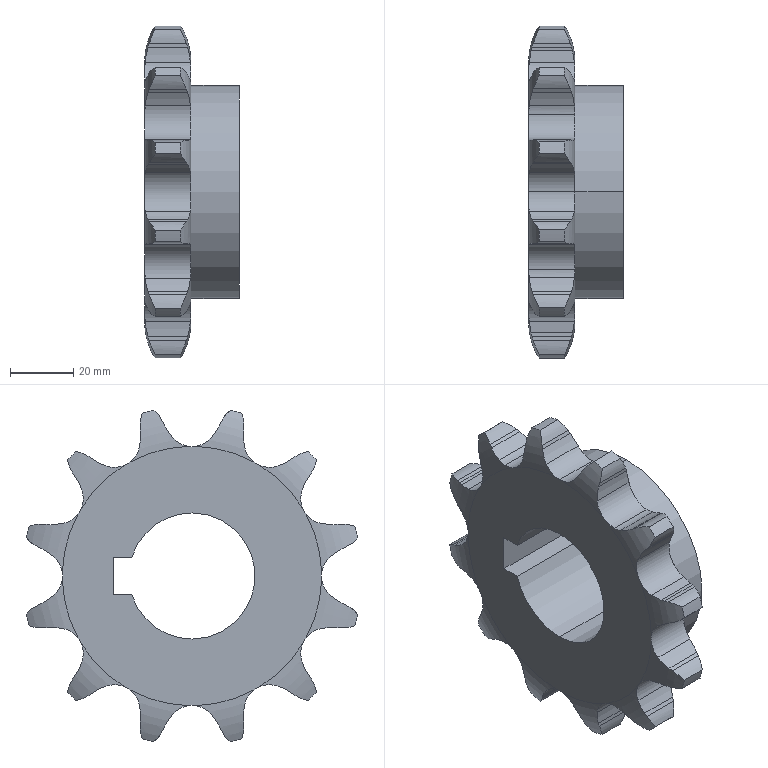Part | STEP file | 1 solid | 138 faces | box 30.002 x 105.245 x 105.245 mm | volume 111853 mm3 | cylinder 84 | plane 30 | torus 24 | commonest cylinder face diameters 23.691 x26 41.467 x26 16.059 x15 108 x12 40 x3 67.629 x2